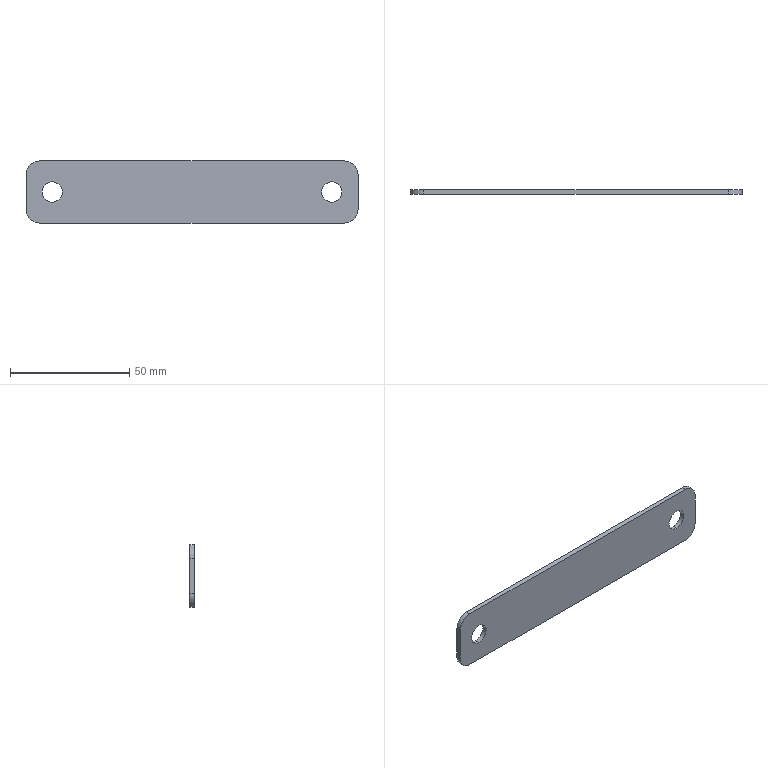Part | STEP file | upcnat117_2_03 | 1 solid | 14 faces | box 139 x 2 x 26 mm | volume 6946 mm3 | cylinder 8 | plane 6 | commonest cylinder face diameters 8.5 x4 11.333 x4
STEP:
#1=CARTESIAN_POINT('',(0.,0.,0.));
#2=DIRECTION('',(0.,0.,1.));
#3=DIRECTION('',(1.,0.,0.));
#4=AXIS2_PLACEMENT_3D('',#1,#2,#3);
#5=CARTESIAN_POINT('',(-58.5,2.,-4.25));
#6=VERTEX_POINT('',#5);
#7=CARTESIAN_POINT('',(-58.5,0.,-4.25));
#8=VERTEX_POINT('',#7);
#9=CARTESIAN_POINT('',(-58.5,0.,-4.25));
#10=DIRECTION('',(0.,-1.,0.));
#11=VECTOR('',#10,1.);
#12=LINE('',#9,#11);
#13=CARTESIAN_POINT('',(-58.5,0.,0.));
#14=DIRECTION('',(0.,-1.,0.));
#15=DIRECTION('',(0.,0.,-1.));
#16=AXIS2_PLACEMENT_3D('',#13,#14,#15);
#17=CYLINDRICAL_SURFACE('',#16,4.25);
#18=CARTESIAN_POINT('',(6.283,0.));
#19=DIRECTION('',(0.,1.));
#20=VECTOR('',#19,1.);
#21=LINE('',#18,#20);
#22=(GEOMETRIC_REPRESENTATION_CONTEXT(2)PARAMETRIC_REPRESENTATION_CONTEXT()REPRESENTATION_CONTEXT('',''));
#23=DEFINITIONAL_REPRESENTATION('',(#21),#22);
#24=PCURVE('',#17,#23);
#25=CARTESIAN_POINT('',(-58.5,0.,0.));
#26=DIRECTION('',(0.,-1.,0.));
#27=DIRECTION('',(0.,0.,-1.));
#28=AXIS2_PLACEMENT_3D('',#25,#26,#27);
#29=CYLINDRICAL_SURFACE('',#28,4.25);
#30=CARTESIAN_POINT('',(0.,0.));
#31=DIRECTION('',(0.,1.));
#32=VECTOR('',#31,1.);
#33=LINE('',#30,#32);
#34=(GEOMETRIC_REPRESENTATION_CONTEXT(2)PARAMETRIC_REPRESENTATION_CONTEXT()REPRESENTATION_CONTEXT('',''));
#35=DEFINITIONAL_REPRESENTATION('',(#33),#34);
#36=PCURVE('',#29,#35);
#37=SURFACE_CURVE('',#12,(#24,#36),.PCURVE_S1.);
#38=EDGE_CURVE('',#6,#8,#37,.T.);
#39=ORIENTED_EDGE('',*,*,#38,.T.);
#40=CARTESIAN_POINT('',(-58.5,0.,4.25));
#41=VERTEX_POINT('',#40);
#42=CARTESIAN_POINT('',(-58.5,0.,0.));
#43=DIRECTION('',(0.,1.,0.));
#44=DIRECTION('',(0.,0.,-1.));
#45=AXIS2_PLACEMENT_3D('',#42,#43,#44);
#46=CIRCLE('',#45,4.25);
#47=CARTESIAN_POINT('',(6.283,0.));
#48=DIRECTION('',(-1.,0.));
#49=VECTOR('',#48,1.);
#50=LINE('',#47,#49);
#51=(GEOMETRIC_REPRESENTATION_CONTEXT(2)PARAMETRIC_REPRESENTATION_CONTEXT()REPRESENTATION_CONTEXT('',''));
#52=DEFINITIONAL_REPRESENTATION('',(#50),#51);
#53=PCURVE('',#17,#52);
#54=CARTESIAN_POINT('',(0.,0.,0.));
#55=DIRECTION('',(0.,1.,0.));
#56=DIRECTION('',(0.,0.,1.));
#57=AXIS2_PLACEMENT_3D('',#54,#55,#56);
#58=PLANE('',#57);
#59=CARTESIAN_POINT('',(0.,-58.5));
#60=DIRECTION('',(-1.,0.));
#61=AXIS2_PLACEMENT_2D('',#59,#60);
#62=CIRCLE('',#61,4.25);
#63=(GEOMETRIC_REPRESENTATION_CONTEXT(2)PARAMETRIC_REPRESENTATION_CONTEXT()REPRESENTATION_CONTEXT('',''));
#64=DEFINITIONAL_REPRESENTATION('',(#62),#63);
#65=PCURVE('',#58,#64);
#66=SURFACE_CURVE('',#46,(#53,#65),.PCURVE_S1.);
#67=EDGE_CURVE('',#8,#41,#66,.T.);
#68=ORIENTED_EDGE('',*,*,#67,.T.);
#69=CARTESIAN_POINT('',(-58.5,2.,4.25));
#70=VERTEX_POINT('',#69);
#71=CARTESIAN_POINT('',(-58.5,0.,4.25));
#72=DIRECTION('',(0.,-1.,0.));
#73=VECTOR('',#72,1.);
#74=LINE('',#71,#73);
#75=CARTESIAN_POINT('',(3.142,0.));
#76=DIRECTION('',(0.,1.));
#77=VECTOR('',#76,1.);
#78=LINE('',#75,#77);
#79=(GEOMETRIC_REPRESENTATION_CONTEXT(2)PARAMETRIC_REPRESENTATION_CONTEXT()REPRESENTATION_CONTEXT('',''));
#80=DEFINITIONAL_REPRESENTATION('',(#78),#79);
#81=PCURVE('',#17,#80);
#82=CARTESIAN_POINT('',(3.142,0.));
#83=DIRECTION('',(0.,1.));
#84=VECTOR('',#83,1.);
#85=LINE('',#82,#84);
#86=(GEOMETRIC_REPRESENTATION_CONTEXT(2)PARAMETRIC_REPRESENTATION_CONTEXT()REPRESENTATION_CONTEXT('',''));
#87=DEFINITIONAL_REPRESENTATION('',(#85),#86);
#88=PCURVE('',#29,#87);
#89=SURFACE_CURVE('',#74,(#81,#88),.PCURVE_S1.);
#90=EDGE_CURVE('',#70,#41,#89,.T.);
#91=ORIENTED_EDGE('',*,*,#90,.F.);
#92=CARTESIAN_POINT('',(-58.5,2.,0.));
#93=DIRECTION('',(0.,-1.,0.));
#94=DIRECTION('',(0.,0.,-1.));
#95=AXIS2_PLACEMENT_3D('',#92,#93,#94);
#96=CIRCLE('',#95,4.25);
#97=CARTESIAN_POINT('',(0.,-2.));
#98=DIRECTION('',(1.,0.));
#99=VECTOR('',#98,1.);
#100=LINE('',#97,#99);
#101=(GEOMETRIC_REPRESENTATION_CONTEXT(2)PARAMETRIC_REPRESENTATION_CONTEXT()REPRESENTATION_CONTEXT('',''));
#102=DEFINITIONAL_REPRESENTATION('',(#100),#101);
#103=PCURVE('',#17,#102);
#104=CARTESIAN_POINT('',(0.,2.,0.));
#105=DIRECTION('',(0.,1.,0.));
#106=DIRECTION('',(0.,0.,1.));
#107=AXIS2_PLACEMENT_3D('',#104,#105,#106);
#108=PLANE('',#107);
#109=CARTESIAN_POINT('',(-4.25,-58.5));
#110=CARTESIAN_POINT('',(-4.25,-51.139));
#111=CARTESIAN_POINT('',(2.125,-54.819));
#112=CARTESIAN_POINT('',(8.5,-58.5));
#113=CARTESIAN_POINT('',(2.125,-62.181));
#114=CARTESIAN_POINT('',(-4.25,-65.861));
#115=CARTESIAN_POINT('',(-4.25,-58.5));
#116=(BOUNDED_CURVE()B_SPLINE_CURVE(2,(#109,#110,#111,#112,#113,#114,#115),.UNSPECIFIED.,.T.,.F.)B_SPLINE_CURVE_WITH_KNOTS((1,2,2,2,2,1),(-2.094,0.,2.094,4.189,6.283,8.378),.UNSPECIFIED.)CURVE()GEOMETRIC_REPRESENTATION_ITEM()RATIONAL_B_SPLINE_CURVE((1.,0.5,1.,0.5,1.,0.5,1.))REPRESENTATION_ITEM(''));
#117=(GEOMETRIC_REPRESENTATION_CONTEXT(2)PARAMETRIC_REPRESENTATION_CONTEXT()REPRESENTATION_CONTEXT('',''));
#118=DEFINITIONAL_REPRESENTATION('',(#116),#117);
#119=PCURVE('',#108,#118);
#120=SURFACE_CURVE('',#96,(#103,#119),.PCURVE_S1.);
#121=EDGE_CURVE('',#70,#6,#120,.T.);
#122=ORIENTED_EDGE('',*,*,#121,.T.);
#123=EDGE_LOOP('',(#39,#68,#91,#122));
#124=FACE_BOUND('',#123,.F.);
#125=ADVANCED_FACE('',(#124),#17,.F.);
#126=CARTESIAN_POINT('',(58.5,2.,-4.25));
#127=VERTEX_POINT('',#126);
#128=CARTESIAN_POINT('',(58.5,0.,-4.25));
#129=VERTEX_POINT('',#128);
#130=CARTESIAN_POINT('',(58.5,0.,-4.25));
#131=DIRECTION('',(0.,-1.,0.));
#132=VECTOR('',#131,1.);
#133=LINE('',#130,#132);
#134=CARTESIAN_POINT('',(58.5,0.,0.));
#135=DIRECTION('',(0.,-1.,0.));
#136=DIRECTION('',(0.,0.,-1.));
#137=AXIS2_PLACEMENT_3D('',#134,#135,#136);
#138=CYLINDRICAL_SURFACE('',#137,4.25);
#139=CARTESIAN_POINT('',(6.283,0.));
#140=DIRECTION('',(0.,1.));
#141=VECTOR('',#140,1.);
#142=LINE('',#139,#141);
#143=(GEOMETRIC_REPRESENTATION_CONTEXT(2)PARAMETRIC_REPRESENTATION_CONTEXT()REPRESENTATION_CONTEXT('',''));
#144=DEFINITIONAL_REPRESENTATION('',(#142),#143);
#145=PCURVE('',#138,#144);
#146=CARTESIAN_POINT('',(58.5,0.,0.));
#147=DIRECTION('',(0.,-1.,0.));
#148=DIRECTION('',(0.,0.,-1.));
#149=AXIS2_PLACEMENT_3D('',#146,#147,#148);
#150=CYLINDRICAL_SURFACE('',#149,4.25);
#151=CARTESIAN_POINT('',(0.,0.));
#152=DIRECTION('',(0.,1.));
#153=VECTOR('',#152,1.);
#154=LINE('',#151,#153);
#155=(GEOMETRIC_REPRESENTATION_CONTEXT(2)PARAMETRIC_REPRESENTATION_CONTEXT()REPRESENTATION_CONTEXT('',''));
#156=DEFINITIONAL_REPRESENTATION('',(#154),#155);
#157=PCURVE('',#150,#156);
#158=SURFACE_CURVE('',#133,(#145,#157),.PCURVE_S1.);
#159=EDGE_CURVE('',#127,#129,#158,.T.);
#160=ORIENTED_EDGE('',*,*,#159,.T.);
#161=CARTESIAN_POINT('',(58.5,0.,4.25));
#162=VERTEX_POINT('',#161);
#163=CARTESIAN_POINT('',(58.5,0.,0.));
#164=DIRECTION('',(0.,1.,0.));
#165=DIRECTION('',(0.,0.,-1.));
#166=AXIS2_PLACEMENT_3D('',#163,#164,#165);
#167=CIRCLE('',#166,4.25);
#168=CARTESIAN_POINT('',(6.283,0.));
#169=DIRECTION('',(-1.,0.));
#170=VECTOR('',#169,1.);
#171=LINE('',#168,#170);
#172=(GEOMETRIC_REPRESENTATION_CONTEXT(2)PARAMETRIC_REPRESENTATION_CONTEXT()REPRESENTATION_CONTEXT('',''));
#173=DEFINITIONAL_REPRESENTATION('',(#171),#172);
#174=PCURVE('',#138,#173);
#175=CARTESIAN_POINT('',(0.,58.5));
#176=DIRECTION('',(-1.,0.));
#177=AXIS2_PLACEMENT_2D('',#175,#176);
#178=CIRCLE('',#177,4.25);
#179=(GEOMETRIC_REPRESENTATION_CONTEXT(2)PARAMETRIC_REPRESENTATION_CONTEXT()REPRESENTATION_CONTEXT('',''));
#180=DEFINITIONAL_REPRESENTATION('',(#178),#179);
#181=PCURVE('',#58,#180);
#182=SURFACE_CURVE('',#167,(#174,#181),.PCURVE_S1.);
#183=EDGE_CURVE('',#129,#162,#182,.T.);
#184=ORIENTED_EDGE('',*,*,#183,.T.);
#185=CARTESIAN_POINT('',(58.5,2.,4.25));
#186=VERTEX_POINT('',#185);
#187=CARTESIAN_POINT('',(58.5,0.,4.25));
#188=DIRECTION('',(0.,-1.,0.));
#189=VECTOR('',#188,1.);
#190=LINE('',#187,#189);
#191=CARTESIAN_POINT('',(3.142,0.));
#192=DIRECTION('',(0.,1.));
#193=VECTOR('',#192,1.);
#194=LINE('',#191,#193);
#195=(GEOMETRIC_REPRESENTATION_CONTEXT(2)PARAMETRIC_REPRESENTATION_CONTEXT()REPRESENTATION_CONTEXT('',''));
#196=DEFINITIONAL_REPRESENTATION('',(#194),#195);
#197=PCURVE('',#138,#196);
#198=CARTESIAN_POINT('',(3.142,0.));
#199=DIRECTION('',(0.,1.));
#200=VECTOR('',#199,1.);
#201=LINE('',#198,#200);
#202=(GEOMETRIC_REPRESENTATION_CONTEXT(2)PARAMETRIC_REPRESENTATION_CONTEXT()REPRESENTATION_CONTEXT('',''));
#203=DEFINITIONAL_REPRESENTATION('',(#201),#202);
#204=PCURVE('',#150,#203);
#205=SURFACE_CURVE('',#190,(#197,#204),.PCURVE_S1.);
#206=EDGE_CURVE('',#186,#162,#205,.T.);
#207=ORIENTED_EDGE('',*,*,#206,.F.);
#208=CARTESIAN_POINT('',(58.5,2.,0.));
#209=DIRECTION('',(0.,-1.,0.));
#210=DIRECTION('',(0.,0.,-1.));
#211=AXIS2_PLACEMENT_3D('',#208,#209,#210);
#212=CIRCLE('',#211,4.25);
#213=CARTESIAN_POINT('',(0.,-2.));
#214=DIRECTION('',(1.,0.));
#215=VECTOR('',#214,1.);
#216=LINE('',#213,#215);
#217=(GEOMETRIC_REPRESENTATION_CONTEXT(2)PARAMETRIC_REPRESENTATION_CONTEXT()REPRESENTATION_CONTEXT('',''));
#218=DEFINITIONAL_REPRESENTATION('',(#216),#217);
#219=PCURVE('',#138,#218);
#220=CARTESIAN_POINT('',(-4.25,58.5));
#221=CARTESIAN_POINT('',(-4.25,65.861));
#222=CARTESIAN_POINT('',(2.125,62.181));
#223=CARTESIAN_POINT('',(8.5,58.5));
#224=CARTESIAN_POINT('',(2.125,54.819));
#225=CARTESIAN_POINT('',(-4.25,51.139));
#226=CARTESIAN_POINT('',(-4.25,58.5));
#227=(BOUNDED_CURVE()B_SPLINE_CURVE(2,(#220,#221,#222,#223,#224,#225,#226),.UNSPECIFIED.,.T.,.F.)B_SPLINE_CURVE_WITH_KNOTS((1,2,2,2,2,1),(-2.094,0.,2.094,4.189,6.283,8.378),.UNSPECIFIED.)CURVE()GEOMETRIC_REPRESENTATION_ITEM()RATIONAL_B_SPLINE_CURVE((1.,0.5,1.,0.5,1.,0.5,1.))REPRESENTATION_ITEM(''));
#228=(GEOMETRIC_REPRESENTATION_CONTEXT(2)PARAMETRIC_REPRESENTATION_CONTEXT()REPRESENTATION_CONTEXT('',''));
#229=DEFINITIONAL_REPRESENTATION('',(#227),#228);
#230=PCURVE('',#108,#229);
#231=SURFACE_CURVE('',#212,(#219,#230),.PCURVE_S1.);
#232=EDGE_CURVE('',#186,#127,#231,.T.);
#233=ORIENTED_EDGE('',*,*,#232,.T.);
#234=EDGE_LOOP('',(#160,#184,#207,#233));
#235=FACE_BOUND('',#234,.F.);
#236=ADVANCED_FACE('',(#235),#138,.F.);
#237=CARTESIAN_POINT('',(-58.5,2.,0.));
#238=DIRECTION('',(0.,-1.,0.));
#239=DIRECTION('',(0.,0.,-1.));
#240=AXIS2_PLACEMENT_3D('',#237,#238,#239);
#241=CIRCLE('',#240,4.25);
#242=CARTESIAN_POINT('',(-4.25,-58.5));
#243=CARTESIAN_POINT('',(-4.25,-51.139));
#244=CARTESIAN_POINT('',(2.125,-54.819));
#245=CARTESIAN_POINT('',(8.5,-58.5));
#246=CARTESIAN_POINT('',(2.125,-62.181));
#247=CARTESIAN_POINT('',(-4.25,-65.861));
#248=CARTESIAN_POINT('',(-4.25,-58.5));
#249=(BOUNDED_CURVE()B_SPLINE_CURVE(2,(#242,#243,#244,#245,#246,#247,#248),.UNSPECIFIED.,.T.,.F.)B_SPLINE_CURVE_WITH_KNOTS((1,2,2,2,2,1),(-2.094,0.,2.094,4.189,6.283,8.378),.UNSPECIFIED.)CURVE()GEOMETRIC_REPRESENTATION_ITEM()RATIONAL_B_SPLINE_CURVE((1.,0.5,1.,0.5,1.,0.5,1.))REPRESENTATION_ITEM(''));
#250=(GEOMETRIC_REPRESENTATION_CONTEXT(2)PARAMETRIC_REPRESENTATION_CONTEXT()REPRESENTATION_CONTEXT('',''));
#251=DEFINITIONAL_REPRESENTATION('',(#249),#250);
#252=PCURVE('',#108,#251);
#253=CARTESIAN_POINT('',(0.,-2.));
#254=DIRECTION('',(1.,0.));
#255=VECTOR('',#254,1.);
#256=LINE('',#253,#255);
#257=(GEOMETRIC_REPRESENTATION_CONTEXT(2)PARAMETRIC_REPRESENTATION_CONTEXT()REPRESENTATION_CONTEXT('',''));
#258=DEFINITIONAL_REPRESENTATION('',(#256),#257);
#259=PCURVE('',#29,#258);
#260=SURFACE_CURVE('',#241,(#252,#259),.PCURVE_S1.);
#261=EDGE_CURVE('',#6,#70,#260,.T.);
#262=ORIENTED_EDGE('',*,*,#261,.T.);
#263=ORIENTED_EDGE('',*,*,#121,.T.);
#264=EDGE_LOOP('',(#262,#263));
#265=FACE_BOUND('',#264,.T.);
#266=CARTESIAN_POINT('',(58.5,2.,0.));
#267=DIRECTION('',(0.,-1.,0.));
#268=DIRECTION('',(0.,0.,-1.));
#269=AXIS2_PLACEMENT_3D('',#266,#267,#268);
#270=CIRCLE('',#269,4.25);
#271=CARTESIAN_POINT('',(-4.25,58.5));
#272=CARTESIAN_POINT('',(-4.25,65.861));
#273=CARTESIAN_POINT('',(2.125,62.181));
#274=CARTESIAN_POINT('',(8.5,58.5));
#275=CARTESIAN_POINT('',(2.125,54.819));
#276=CARTESIAN_POINT('',(-4.25,51.139));
#277=CARTESIAN_POINT('',(-4.25,58.5));
#278=(BOUNDED_CURVE()B_SPLINE_CURVE(2,(#271,#272,#273,#274,#275,#276,#277),.UNSPECIFIED.,.T.,.F.)B_SPLINE_CURVE_WITH_KNOTS((1,2,2,2,2,1),(-2.094,0.,2.094,4.189,6.283,8.378),.UNSPECIFIED.)CURVE()GEOMETRIC_REPRESENTATION_ITEM()RATIONAL_B_SPLINE_CURVE((1.,0.5,1.,0.5,1.,0.5,1.))REPRESENTATION_ITEM(''));
#279=(GEOMETRIC_REPRESENTATION_CONTEXT(2)PARAMETRIC_REPRESENTATION_CONTEXT()REPRESENTATION_CONTEXT('',''));
#280=DEFINITIONAL_REPRESENTATION('',(#278),#279);
#281=PCURVE('',#108,#280);
#282=CARTESIAN_POINT('',(0.,-2.));
#283=DIRECTION('',(1.,0.));
#284=VECTOR('',#283,1.);
#285=LINE('',#282,#284);
#286=(GEOMETRIC_REPRESENTATION_CONTEXT(2)PARAMETRIC_REPRESENTATION_CONTEXT()REPRESENTATION_CONTEXT('',''));
#287=DEFINITIONAL_REPRESENTATION('',(#285),#286);
#288=PCURVE('',#150,#287);
#289=SURFACE_CURVE('',#270,(#281,#288),.PCURVE_S1.);
#290=EDGE_CURVE('',#127,#186,#289,.T.);
#291=ORIENTED_EDGE('',*,*,#290,.T.);
#292=ORIENTED_EDGE('',*,*,#232,.T.);
#293=EDGE_LOOP('',(#291,#292));
#294=FACE_BOUND('',#293,.T.);
#295=CARTESIAN_POINT('',(63.833,2.,-13.));
#296=VERTEX_POINT('',#295);
#297=CARTESIAN_POINT('',(-63.833,2.,-13.));
#298=VERTEX_POINT('',#297);
#299=CARTESIAN_POINT('',(0.,2.,-13.));
#300=DIRECTION('',(-1.,0.,0.));
#301=VECTOR('',#300,1.);
#302=LINE('',#299,#301);
#303=CARTESIAN_POINT('',(-13.,0.));
#304=DIRECTION('',(0.,-1.));
#305=VECTOR('',#304,1.);
#306=LINE('',#303,#305);
#307=(GEOMETRIC_REPRESENTATION_CONTEXT(2)PARAMETRIC_REPRESENTATION_CONTEXT()REPRESENTATION_CONTEXT('',''));
#308=DEFINITIONAL_REPRESENTATION('',(#306),#307);
#309=PCURVE('',#108,#308);
#310=CARTESIAN_POINT('',(-63.833,0.,-13.));
#311=DIRECTION('',(0.,0.,-1.));
#312=DIRECTION('',(-1.,0.,0.));
#313=AXIS2_PLACEMENT_3D('',#310,#311,#312);
#314=PLANE('',#313);
#315=CARTESIAN_POINT('',(-63.833,2.));
#316=DIRECTION('',(1.,0.));
#317=VECTOR('',#316,1.);
#318=LINE('',#315,#317);
#319=(GEOMETRIC_REPRESENTATION_CONTEXT(2)PARAMETRIC_REPRESENTATION_CONTEXT()REPRESENTATION_CONTEXT('',''));
#320=DEFINITIONAL_REPRESENTATION('',(#318),#319);
#321=PCURVE('',#314,#320);
#322=SURFACE_CURVE('',#302,(#309,#321),.PCURVE_S1.);
#323=EDGE_CURVE('',#296,#298,#322,.T.);
#324=ORIENTED_EDGE('',*,*,#323,.T.);
#325=CARTESIAN_POINT('',(-69.5,2.,-7.333));
#326=VERTEX_POINT('',#325);
#327=CARTESIAN_POINT('',(-63.833,2.,-7.333));
#328=DIRECTION('',(0.,1.,0.));
#329=DIRECTION('',(0.,0.,-1.));
#330=AXIS2_PLACEMENT_3D('',#327,#328,#329);
#331=CIRCLE('',#330,5.667);
#332=CARTESIAN_POINT('',(-7.333,-63.833));
#333=DIRECTION('',(-1.,0.));
#334=AXIS2_PLACEMENT_2D('',#332,#333);
#335=CIRCLE('',#334,5.667);
#336=(GEOMETRIC_REPRESENTATION_CONTEXT(2)PARAMETRIC_REPRESENTATION_CONTEXT()REPRESENTATION_CONTEXT('',''));
#337=DEFINITIONAL_REPRESENTATION('',(#335),#336);
#338=PCURVE('',#108,#337);
#339=CARTESIAN_POINT('',(-63.833,0.,-7.333));
#340=DIRECTION('',(0.,-1.,0.));
#341=DIRECTION('',(0.,0.,-1.));
#342=AXIS2_PLACEMENT_3D('',#339,#340,#341);
#343=CYLINDRICAL_SURFACE('',#342,5.667);
#344=CARTESIAN_POINT('',(6.283,-2.));
#345=DIRECTION('',(-1.,0.));
#346=VECTOR('',#345,1.);
#347=LINE('',#344,#346);
#348=(GEOMETRIC_REPRESENTATION_CONTEXT(2)PARAMETRIC_REPRESENTATION_CONTEXT()REPRESENTATION_CONTEXT('',''));
#349=DEFINITIONAL_REPRESENTATION('',(#347),#348);
#350=PCURVE('',#343,#349);
#351=SURFACE_CURVE('',#331,(#338,#350),.PCURVE_S1.);
#352=EDGE_CURVE('',#298,#326,#351,.T.);
#353=ORIENTED_EDGE('',*,*,#352,.T.);
#354=CARTESIAN_POINT('',(-69.5,2.,7.333));
#355=VERTEX_POINT('',#354);
#356=CARTESIAN_POINT('',(-69.5,2.,0.));
#357=DIRECTION('',(0.,0.,1.));
#358=VECTOR('',#357,1.);
#359=LINE('',#356,#358);
#360=CARTESIAN_POINT('',(0.,-69.5));
#361=DIRECTION('',(1.,0.));
#362=VECTOR('',#361,1.);
#363=LINE('',#360,#362);
#364=(GEOMETRIC_REPRESENTATION_CONTEXT(2)PARAMETRIC_REPRESENTATION_CONTEXT()REPRESENTATION_CONTEXT('',''));
#365=DEFINITIONAL_REPRESENTATION('',(#363),#364);
#366=PCURVE('',#108,#365);
#367=CARTESIAN_POINT('',(-69.5,0.,7.333));
#368=DIRECTION('',(-1.,0.,0.));
#369=DIRECTION('',(0.,0.,1.));
#370=AXIS2_PLACEMENT_3D('',#367,#368,#369);
#371=PLANE('',#370);
#372=CARTESIAN_POINT('',(-7.333,2.));
#373=DIRECTION('',(1.,0.));
#374=VECTOR('',#373,1.);
#375=LINE('',#372,#374);
#376=(GEOMETRIC_REPRESENTATION_CONTEXT(2)PARAMETRIC_REPRESENTATION_CONTEXT()REPRESENTATION_CONTEXT('',''));
#377=DEFINITIONAL_REPRESENTATION('',(#375),#376);
#378=PCURVE('',#371,#377);
#379=SURFACE_CURVE('',#359,(#366,#378),.PCURVE_S1.);
#380=EDGE_CURVE('',#326,#355,#379,.T.);
#381=ORIENTED_EDGE('',*,*,#380,.T.);
#382=CARTESIAN_POINT('',(-63.833,2.,13.));
#383=VERTEX_POINT('',#382);
#384=CARTESIAN_POINT('',(-63.833,2.,7.333));
#385=DIRECTION('',(0.,1.,0.));
#386=DIRECTION('',(0.,0.,-1.));
#387=AXIS2_PLACEMENT_3D('',#384,#385,#386);
#388=CIRCLE('',#387,5.667);
#389=CARTESIAN_POINT('',(7.333,-63.833));
#390=DIRECTION('',(-1.,0.));
#391=AXIS2_PLACEMENT_2D('',#389,#390);
#392=CIRCLE('',#391,5.667);
#393=(GEOMETRIC_REPRESENTATION_CONTEXT(2)PARAMETRIC_REPRESENTATION_CONTEXT()REPRESENTATION_CONTEXT('',''));
#394=DEFINITIONAL_REPRESENTATION('',(#392),#393);
#395=PCURVE('',#108,#394);
#396=CARTESIAN_POINT('',(-63.833,0.,7.333));
#397=DIRECTION('',(0.,-1.,0.));
#398=DIRECTION('',(0.,0.,-1.));
#399=AXIS2_PLACEMENT_3D('',#396,#397,#398);
#400=CYLINDRICAL_SURFACE('',#399,5.667);
#401=CARTESIAN_POINT('',(6.283,-2.));
#402=DIRECTION('',(-1.,0.));
#403=VECTOR('',#402,1.);
#404=LINE('',#401,#403);
#405=(GEOMETRIC_REPRESENTATION_CONTEXT(2)PARAMETRIC_REPRESENTATION_CONTEXT()REPRESENTATION_CONTEXT('',''));
#406=DEFINITIONAL_REPRESENTATION('',(#404),#405);
#407=PCURVE('',#400,#406);
#408=SURFACE_CURVE('',#388,(#395,#407),.PCURVE_S1.);
#409=EDGE_CURVE('',#355,#383,#408,.T.);
#410=ORIENTED_EDGE('',*,*,#409,.T.);
#411=CARTESIAN_POINT('',(63.833,2.,13.));
#412=VERTEX_POINT('',#411);
#413=CARTESIAN_POINT('',(0.,2.,13.));
#414=DIRECTION('',(1.,0.,0.));
#415=VECTOR('',#414,1.);
#416=LINE('',#413,#415);
#417=CARTESIAN_POINT('',(13.,0.));
#418=DIRECTION('',(0.,1.));
#419=VECTOR('',#418,1.);
#420=LINE('',#417,#419);
#421=(GEOMETRIC_REPRESENTATION_CONTEXT(2)PARAMETRIC_REPRESENTATION_CONTEXT()REPRESENTATION_CONTEXT('',''));
#422=DEFINITIONAL_REPRESENTATION('',(#420),#421);
#423=PCURVE('',#108,#422);
#424=CARTESIAN_POINT('',(63.833,0.,13.));
#425=DIRECTION('',(0.,0.,1.));
#426=DIRECTION('',(1.,0.,0.));
#427=AXIS2_PLACEMENT_3D('',#424,#425,#426);
#428=PLANE('',#427);
#429=CARTESIAN_POINT('',(-63.833,2.));
#430=DIRECTION('',(1.,0.));
#431=VECTOR('',#430,1.);
#432=LINE('',#429,#431);
#433=(GEOMETRIC_REPRESENTATION_CONTEXT(2)PARAMETRIC_REPRESENTATION_CONTEXT()REPRESENTATION_CONTEXT('',''));
#434=DEFINITIONAL_REPRESENTATION('',(#432),#433);
#435=PCURVE('',#428,#434);
#436=SURFACE_CURVE('',#416,(#423,#435),.PCURVE_S1.);
#437=EDGE_CURVE('',#383,#412,#436,.T.);
#438=ORIENTED_EDGE('',*,*,#437,.T.);
#439=CARTESIAN_POINT('',(69.5,2.,7.333));
#440=VERTEX_POINT('',#439);
#441=CARTESIAN_POINT('',(63.833,2.,7.333));
#442=DIRECTION('',(0.,1.,0.));
#443=DIRECTION('',(0.,0.,-1.));
#444=AXIS2_PLACEMENT_3D('',#441,#442,#443);
#445=CIRCLE('',#444,5.667);
#446=CARTESIAN_POINT('',(7.333,63.833));
#447=DIRECTION('',(-1.,0.));
#448=AXIS2_PLACEMENT_2D('',#446,#447);
#449=CIRCLE('',#448,5.667);
#450=(GEOMETRIC_REPRESENTATION_CONTEXT(2)PARAMETRIC_REPRESENTATION_CONTEXT()REPRESENTATION_CONTEXT('',''));
#451=DEFINITIONAL_REPRESENTATION('',(#449),#450);
#452=PCURVE('',#108,#451);
#453=CARTESIAN_POINT('',(63.833,0.,7.333));
#454=DIRECTION('',(0.,-1.,0.));
#455=DIRECTION('',(0.,0.,-1.));
#456=AXIS2_PLACEMENT_3D('',#453,#454,#455);
#457=CYLINDRICAL_SURFACE('',#456,5.667);
#458=CARTESIAN_POINT('',(6.283,-2.));
#459=DIRECTION('',(-1.,0.));
#460=VECTOR('',#459,1.);
#461=LINE('',#458,#460);
#462=(GEOMETRIC_REPRESENTATION_CONTEXT(2)PARAMETRIC_REPRESENTATION_CONTEXT()REPRESENTATION_CONTEXT('',''));
#463=DEFINITIONAL_REPRESENTATION('',(#461),#462);
#464=PCURVE('',#457,#463);
#465=SURFACE_CURVE('',#445,(#452,#464),.PCURVE_S1.);
#466=EDGE_CURVE('',#412,#440,#465,.T.);
#467=ORIENTED_EDGE('',*,*,#466,.T.);
#468=CARTESIAN_POINT('',(69.5,2.,-7.333));
#469=VERTEX_POINT('',#468);
#470=CARTESIAN_POINT('',(69.5,2.,0.));
#471=DIRECTION('',(0.,0.,-1.));
#472=VECTOR('',#471,1.);
#473=LINE('',#470,#472);
#474=CARTESIAN_POINT('',(0.,69.5));
#475=DIRECTION('',(-1.,0.));
#476=VECTOR('',#475,1.);
#477=LINE('',#474,#476);
#478=(GEOMETRIC_REPRESENTATION_CONTEXT(2)PARAMETRIC_REPRESENTATION_CONTEXT()REPRESENTATION_CONTEXT('',''));
#479=DEFINITIONAL_REPRESENTATION('',(#477),#478);
#480=PCURVE('',#108,#479);
#481=CARTESIAN_POINT('',(69.5,0.,-7.333));
#482=DIRECTION('',(1.,0.,0.));
#483=DIRECTION('',(0.,0.,-1.));
#484=AXIS2_PLACEMENT_3D('',#481,#482,#483);
#485=PLANE('',#484);
#486=CARTESIAN_POINT('',(-7.333,2.));
#487=DIRECTION('',(1.,0.));
#488=VECTOR('',#487,1.);
#489=LINE('',#486,#488);
#490=(GEOMETRIC_REPRESENTATION_CONTEXT(2)PARAMETRIC_REPRESENTATION_CONTEXT()REPRESENTATION_CONTEXT('',''));
#491=DEFINITIONAL_REPRESENTATION('',(#489),#490);
#492=PCURVE('',#485,#491);
#493=SURFACE_CURVE('',#473,(#480,#492),.PCURVE_S1.);
#494=EDGE_CURVE('',#440,#469,#493,.T.);
#495=ORIENTED_EDGE('',*,*,#494,.T.);
#496=CARTESIAN_POINT('',(63.833,2.,-7.333));
#497=DIRECTION('',(0.,1.,0.));
#498=DIRECTION('',(0.,0.,-1.));
#499=AXIS2_PLACEMENT_3D('',#496,#497,#498);
#500=CIRCLE('',#499,5.667);
#501=CARTESIAN_POINT('',(-7.333,63.833));
#502=DIRECTION('',(-1.,0.));
#503=AXIS2_PLACEMENT_2D('',#501,#502);
#504=CIRCLE('',#503,5.667);
#505=(GEOMETRIC_REPRESENTATION_CONTEXT(2)PARAMETRIC_REPRESENTATION_CONTEXT()REPRESENTATION_CONTEXT('',''));
#506=DEFINITIONAL_REPRESENTATION('',(#504),#505);
#507=PCURVE('',#108,#506);
#508=CARTESIAN_POINT('',(63.833,0.,-7.333));
#509=DIRECTION('',(0.,-1.,0.));
#510=DIRECTION('',(0.,0.,-1.));
#511=AXIS2_PLACEMENT_3D('',#508,#509,#510);
#512=CYLINDRICAL_SURFACE('',#511,5.667);
#513=CARTESIAN_POINT('',(6.283,-2.));
#514=DIRECTION('',(-1.,0.));
#515=VECTOR('',#514,1.);
#516=LINE('',#513,#515);
#517=(GEOMETRIC_REPRESENTATION_CONTEXT(2)PARAMETRIC_REPRESENTATION_CONTEXT()REPRESENTATION_CONTEXT('',''));
#518=DEFINITIONAL_REPRESENTATION('',(#516),#517);
#519=PCURVE('',#512,#518);
#520=SURFACE_CURVE('',#500,(#507,#519),.PCURVE_S1.);
#521=EDGE_CURVE('',#469,#296,#520,.T.);
#522=ORIENTED_EDGE('',*,*,#521,.T.);
#523=EDGE_LOOP('',(#324,#353,#381,#410,#438,#467,#495,#522));
#524=FACE_BOUND('',#523,.T.);
#525=ADVANCED_FACE('',(#265,#294,#524),#108,.T.);
#526=CARTESIAN_POINT('',(-58.5,0.,0.));
#527=DIRECTION('',(0.,1.,0.));
#528=DIRECTION('',(0.,0.,-1.));
#529=AXIS2_PLACEMENT_3D('',#526,#527,#528);
#530=CIRCLE('',#529,4.25);
#531=CARTESIAN_POINT('',(6.283,0.));
#532=DIRECTION('',(-1.,0.));
#533=VECTOR('',#532,1.);
#534=LINE('',#531,#533);
#535=(GEOMETRIC_REPRESENTATION_CONTEXT(2)PARAMETRIC_REPRESENTATION_CONTEXT()REPRESENTATION_CONTEXT('',''));
#536=DEFINITIONAL_REPRESENTATION('',(#534),#535);
#537=PCURVE('',#29,#536);
#538=CARTESIAN_POINT('',(0.,-58.5));
#539=DIRECTION('',(-1.,0.));
#540=AXIS2_PLACEMENT_2D('',#538,#539);
#541=CIRCLE('',#540,4.25);
#542=(GEOMETRIC_REPRESENTATION_CONTEXT(2)PARAMETRIC_REPRESENTATION_CONTEXT()REPRESENTATION_CONTEXT('',''));
#543=DEFINITIONAL_REPRESENTATION('',(#541),#542);
#544=PCURVE('',#58,#543);
#545=SURFACE_CURVE('',#530,(#537,#544),.PCURVE_S1.);
#546=EDGE_CURVE('',#41,#8,#545,.T.);
#547=ORIENTED_EDGE('',*,*,#546,.T.);
#548=ORIENTED_EDGE('',*,*,#38,.F.);
#549=ORIENTED_EDGE('',*,*,#261,.T.);
#550=ORIENTED_EDGE('',*,*,#90,.T.);
#551=EDGE_LOOP('',(#547,#548,#549,#550));
#552=FACE_BOUND('',#551,.F.);
#553=ADVANCED_FACE('',(#552),#29,.F.);
#554=CARTESIAN_POINT('',(58.5,0.,0.));
#555=DIRECTION('',(0.,1.,0.));
#556=DIRECTION('',(0.,0.,-1.));
#557=AXIS2_PLACEMENT_3D('',#554,#555,#556);
#558=CIRCLE('',#557,4.25);
#559=CARTESIAN_POINT('',(6.283,0.));
#560=DIRECTION('',(-1.,0.));
#561=VECTOR('',#560,1.);
#562=LINE('',#559,#561);
#563=(GEOMETRIC_REPRESENTATION_CONTEXT(2)PARAMETRIC_REPRESENTATION_CONTEXT()REPRESENTATION_CONTEXT('',''));
#564=DEFINITIONAL_REPRESENTATION('',(#562),#563);
#565=PCURVE('',#150,#564);
#566=CARTESIAN_POINT('',(0.,58.5));
#567=DIRECTION('',(-1.,0.));
#568=AXIS2_PLACEMENT_2D('',#566,#567);
#569=CIRCLE('',#568,4.25);
#570=(GEOMETRIC_REPRESENTATION_CONTEXT(2)PARAMETRIC_REPRESENTATION_CONTEXT()REPRESENTATION_CONTEXT('',''));
#571=DEFINITIONAL_REPRESENTATION('',(#569),#570);
#572=PCURVE('',#58,#571);
#573=SURFACE_CURVE('',#558,(#565,#572),.PCURVE_S1.);
#574=EDGE_CURVE('',#162,#129,#573,.T.);
#575=ORIENTED_EDGE('',*,*,#574,.T.);
#576=ORIENTED_EDGE('',*,*,#159,.F.);
#577=ORIENTED_EDGE('',*,*,#290,.T.);
#578=ORIENTED_EDGE('',*,*,#206,.T.);
#579=EDGE_LOOP('',(#575,#576,#577,#578));
#580=FACE_BOUND('',#579,.F.);
#581=ADVANCED_FACE('',(#580),#150,.F.);
#582=CARTESIAN_POINT('',(-63.833,0.,-13.));
#583=VERTEX_POINT('',#582);
#584=CARTESIAN_POINT('',(-69.5,0.,-7.333));
#585=VERTEX_POINT('',#584);
#586=CARTESIAN_POINT('',(-63.833,0.,-7.333));
#587=DIRECTION('',(0.,1.,0.));
#588=DIRECTION('',(0.,0.,-1.));
#589=AXIS2_PLACEMENT_3D('',#586,#587,#588);
#590=CIRCLE('',#589,5.667);
#591=CARTESIAN_POINT('',(6.283,0.));
#592=DIRECTION('',(-1.,0.));
#593=VECTOR('',#592,1.);
#594=LINE('',#591,#593);
#595=(GEOMETRIC_REPRESENTATION_CONTEXT(2)PARAMETRIC_REPRESENTATION_CONTEXT()REPRESENTATION_CONTEXT('',''));
#596=DEFINITIONAL_REPRESENTATION('',(#594),#595);
#597=PCURVE('',#343,#596);
#598=CARTESIAN_POINT('',(-7.333,-63.833));
#599=DIRECTION('',(-1.,0.));
#600=AXIS2_PLACEMENT_2D('',#598,#599);
#601=CIRCLE('',#600,5.667);
#602=(GEOMETRIC_REPRESENTATION_CONTEXT(2)PARAMETRIC_REPRESENTATION_CONTEXT()REPRESENTATION_CONTEXT('',''));
#603=DEFINITIONAL_REPRESENTATION('',(#601),#602);
#604=PCURVE('',#58,#603);
#605=SURFACE_CURVE('',#590,(#597,#604),.PCURVE_S1.);
#606=EDGE_CURVE('',#583,#585,#605,.T.);
#607=ORIENTED_EDGE('',*,*,#606,.T.);
#608=CARTESIAN_POINT('',(-69.5,0.,-7.333));
#609=DIRECTION('',(0.,1.,0.));
#610=VECTOR('',#609,1.);
#611=LINE('',#608,#610);
#612=CARTESIAN_POINT('',(4.712,0.));
#613=DIRECTION('',(0.,-1.));
#614=VECTOR('',#613,1.);
#615=LINE('',#612,#614);
#616=(GEOMETRIC_REPRESENTATION_CONTEXT(2)PARAMETRIC_REPRESENTATION_CONTEXT()REPRESENTATION_CONTEXT('',''));
#617=DEFINITIONAL_REPRESENTATION('',(#615),#616);
#618=PCURVE('',#343,#617);
#619=CARTESIAN_POINT('',(-14.667,0.));
#620=DIRECTION('',(0.,1.));
#621=VECTOR('',#620,1.);
#622=LINE('',#619,#621);
#623=(GEOMETRIC_REPRESENTATION_CONTEXT(2)PARAMETRIC_REPRESENTATION_CONTEXT()REPRESENTATION_CONTEXT('',''));
#624=DEFINITIONAL_REPRESENTATION('',(#622),#623);
#625=PCURVE('',#371,#624);
#626=SURFACE_CURVE('',#611,(#618,#625),.PCURVE_S1.);
#627=EDGE_CURVE('',#585,#326,#626,.T.);
#628=ORIENTED_EDGE('',*,*,#627,.T.);
#629=ORIENTED_EDGE('',*,*,#352,.F.);
#630=CARTESIAN_POINT('',(-63.833,0.,-13.));
#631=DIRECTION('',(0.,-1.,0.));
#632=VECTOR('',#631,1.);
#633=LINE('',#630,#632);
#634=CARTESIAN_POINT('',(6.283,0.));
#635=DIRECTION('',(0.,1.));
#636=VECTOR('',#635,1.);
#637=LINE('',#634,#636);
#638=(GEOMETRIC_REPRESENTATION_CONTEXT(2)PARAMETRIC_REPRESENTATION_CONTEXT()REPRESENTATION_CONTEXT('',''));
#639=DEFINITIONAL_REPRESENTATION('',(#637),#638);
#640=PCURVE('',#343,#639);
#641=CARTESIAN_POINT('',(0.,0.));
#642=DIRECTION('',(0.,-1.));
#643=VECTOR('',#642,1.);
#644=LINE('',#641,#643);
#645=(GEOMETRIC_REPRESENTATION_CONTEXT(2)PARAMETRIC_REPRESENTATION_CONTEXT()REPRESENTATION_CONTEXT('',''));
#646=DEFINITIONAL_REPRESENTATION('',(#644),#645);
#647=PCURVE('',#314,#646);
#648=SURFACE_CURVE('',#633,(#640,#647),.PCURVE_S1.);
#649=EDGE_CURVE('',#298,#583,#648,.T.);
#650=ORIENTED_EDGE('',*,*,#649,.T.);
#651=EDGE_LOOP('',(#607,#628,#629,#650));
#652=FACE_BOUND('',#651,.T.);
#653=ADVANCED_FACE('',(#652),#343,.T.);
#654=CARTESIAN_POINT('',(63.833,0.,-13.));
#655=VERTEX_POINT('',#654);
#656=CARTESIAN_POINT('',(-63.833,0.,-13.));
#657=DIRECTION('',(-1.,0.,0.));
#658=VECTOR('',#657,1.);
#659=LINE('',#656,#658);
#660=CARTESIAN_POINT('',(0.,0.));
#661=DIRECTION('',(1.,0.));
#662=VECTOR('',#661,1.);
#663=LINE('',#660,#662);
#664=(GEOMETRIC_REPRESENTATION_CONTEXT(2)PARAMETRIC_REPRESENTATION_CONTEXT()REPRESENTATION_CONTEXT('',''));
#665=DEFINITIONAL_REPRESENTATION('',(#663),#664);
#666=PCURVE('',#314,#665);
#667=CARTESIAN_POINT('',(-13.,-63.833));
#668=DIRECTION('',(0.,-1.));
#669=VECTOR('',#668,1.);
#670=LINE('',#667,#669);
#671=(GEOMETRIC_REPRESENTATION_CONTEXT(2)PARAMETRIC_REPRESENTATION_CONTEXT()REPRESENTATION_CONTEXT('',''));
#672=DEFINITIONAL_REPRESENTATION('',(#670),#671);
#673=PCURVE('',#58,#672);
#674=SURFACE_CURVE('',#659,(#666,#673),.PCURVE_S1.);
#675=EDGE_CURVE('',#655,#583,#674,.T.);
#676=ORIENTED_EDGE('',*,*,#675,.T.);
#677=ORIENTED_EDGE('',*,*,#649,.F.);
#678=ORIENTED_EDGE('',*,*,#323,.F.);
#679=CARTESIAN_POINT('',(63.833,0.,-13.));
#680=DIRECTION('',(0.,-1.,0.));
#681=VECTOR('',#680,1.);
#682=LINE('',#679,#681);
#683=CARTESIAN_POINT('',(-127.667,0.));
#684=DIRECTION('',(0.,-1.));
#685=VECTOR('',#684,1.);
#686=LINE('',#683,#685);
#687=(GEOMETRIC_REPRESENTATION_CONTEXT(2)PARAMETRIC_REPRESENTATION_CONTEXT()REPRESENTATION_CONTEXT('',''));
#688=DEFINITIONAL_REPRESENTATION('',(#686),#687);
#689=PCURVE('',#314,#688);
#690=CARTESIAN_POINT('',(0.,0.));
#691=DIRECTION('',(0.,1.));
#692=VECTOR('',#691,1.);
#693=LINE('',#690,#692);
#694=(GEOMETRIC_REPRESENTATION_CONTEXT(2)PARAMETRIC_REPRESENTATION_CONTEXT()REPRESENTATION_CONTEXT('',''));
#695=DEFINITIONAL_REPRESENTATION('',(#693),#694);
#696=PCURVE('',#512,#695);
#697=SURFACE_CURVE('',#682,(#689,#696),.PCURVE_S1.);
#698=EDGE_CURVE('',#296,#655,#697,.T.);
#699=ORIENTED_EDGE('',*,*,#698,.T.);
#700=EDGE_LOOP('',(#676,#677,#678,#699));
#701=FACE_BOUND('',#700,.T.);
#702=ADVANCED_FACE('',(#701),#314,.T.);
#703=CARTESIAN_POINT('',(69.5,0.,-7.333));
#704=VERTEX_POINT('',#703);
#705=CARTESIAN_POINT('',(63.833,0.,-7.333));
#706=DIRECTION('',(0.,1.,0.));
#707=DIRECTION('',(0.,0.,-1.));
#708=AXIS2_PLACEMENT_3D('',#705,#706,#707);
#709=CIRCLE('',#708,5.667);
#710=CARTESIAN_POINT('',(6.283,0.));
#711=DIRECTION('',(-1.,0.));
#712=VECTOR('',#711,1.);
#713=LINE('',#710,#712);
#714=(GEOMETRIC_REPRESENTATION_CONTEXT(2)PARAMETRIC_REPRESENTATION_CONTEXT()REPRESENTATION_CONTEXT('',''));
#715=DEFINITIONAL_REPRESENTATION('',(#713),#714);
#716=PCURVE('',#512,#715);
#717=CARTESIAN_POINT('',(-7.333,63.833));
#718=DIRECTION('',(-1.,0.));
#719=AXIS2_PLACEMENT_2D('',#717,#718);
#720=CIRCLE('',#719,5.667);
#721=(GEOMETRIC_REPRESENTATION_CONTEXT(2)PARAMETRIC_REPRESENTATION_CONTEXT()REPRESENTATION_CONTEXT('',''));
#722=DEFINITIONAL_REPRESENTATION('',(#720),#721);
#723=PCURVE('',#58,#722);
#724=SURFACE_CURVE('',#709,(#716,#723),.PCURVE_S1.);
#725=EDGE_CURVE('',#704,#655,#724,.T.);
#726=ORIENTED_EDGE('',*,*,#725,.T.);
#727=ORIENTED_EDGE('',*,*,#698,.F.);
#728=ORIENTED_EDGE('',*,*,#521,.F.);
#729=CARTESIAN_POINT('',(69.5,0.,-7.333));
#730=DIRECTION('',(0.,-1.,0.));
#731=VECTOR('',#730,1.);
#732=LINE('',#729,#731);
#733=CARTESIAN_POINT('',(1.571,0.));
#734=DIRECTION('',(0.,1.));
#735=VECTOR('',#734,1.);
#736=LINE('',#733,#735);
#737=(GEOMETRIC_REPRESENTATION_CONTEXT(2)PARAMETRIC_REPRESENTATION_CONTEXT()REPRESENTATION_CONTEXT('',''));
#738=DEFINITIONAL_REPRESENTATION('',(#736),#737);
#739=PCURVE('',#512,#738);
#740=CARTESIAN_POINT('',(0.,0.));
#741=DIRECTION('',(0.,-1.));
#742=VECTOR('',#741,1.);
#743=LINE('',#740,#742);
#744=(GEOMETRIC_REPRESENTATION_CONTEXT(2)PARAMETRIC_REPRESENTATION_CONTEXT()REPRESENTATION_CONTEXT('',''));
#745=DEFINITIONAL_REPRESENTATION('',(#743),#744);
#746=PCURVE('',#485,#745);
#747=SURFACE_CURVE('',#732,(#739,#746),.PCURVE_S1.);
#748=EDGE_CURVE('',#469,#704,#747,.T.);
#749=ORIENTED_EDGE('',*,*,#748,.T.);
#750=EDGE_LOOP('',(#726,#727,#728,#749));
#751=FACE_BOUND('',#750,.T.);
#752=ADVANCED_FACE('',(#751),#512,.T.);
#753=CARTESIAN_POINT('',(69.5,0.,7.333));
#754=VERTEX_POINT('',#753);
#755=CARTESIAN_POINT('',(69.5,0.,-7.333));
#756=DIRECTION('',(0.,0.,-1.));
#757=VECTOR('',#756,1.);
#758=LINE('',#755,#757);
#759=CARTESIAN_POINT('',(0.,0.));
#760=DIRECTION('',(1.,0.));
#761=VECTOR('',#760,1.);
#762=LINE('',#759,#761);
#763=(GEOMETRIC_REPRESENTATION_CONTEXT(2)PARAMETRIC_REPRESENTATION_CONTEXT()REPRESENTATION_CONTEXT('',''));
#764=DEFINITIONAL_REPRESENTATION('',(#762),#763);
#765=PCURVE('',#485,#764);
#766=CARTESIAN_POINT('',(-7.333,69.5));
#767=DIRECTION('',(-1.,0.));
#768=VECTOR('',#767,1.);
#769=LINE('',#766,#768);
#770=(GEOMETRIC_REPRESENTATION_CONTEXT(2)PARAMETRIC_REPRESENTATION_CONTEXT()REPRESENTATION_CONTEXT('',''));
#771=DEFINITIONAL_REPRESENTATION('',(#769),#770);
#772=PCURVE('',#58,#771);
#773=SURFACE_CURVE('',#758,(#765,#772),.PCURVE_S1.);
#774=EDGE_CURVE('',#754,#704,#773,.T.);
#775=ORIENTED_EDGE('',*,*,#774,.T.);
#776=ORIENTED_EDGE('',*,*,#748,.F.);
#777=ORIENTED_EDGE('',*,*,#494,.F.);
#778=CARTESIAN_POINT('',(69.5,0.,7.333));
#779=DIRECTION('',(0.,-1.,0.));
#780=VECTOR('',#779,1.);
#781=LINE('',#778,#780);
#782=CARTESIAN_POINT('',(-14.667,0.));
#783=DIRECTION('',(0.,-1.));
#784=VECTOR('',#783,1.);
#785=LINE('',#782,#784);
#786=(GEOMETRIC_REPRESENTATION_CONTEXT(2)PARAMETRIC_REPRESENTATION_CONTEXT()REPRESENTATION_CONTEXT('',''));
#787=DEFINITIONAL_REPRESENTATION('',(#785),#786);
#788=PCURVE('',#485,#787);
#789=CARTESIAN_POINT('',(1.571,0.));
#790=DIRECTION('',(0.,1.));
#791=VECTOR('',#790,1.);
#792=LINE('',#789,#791);
#793=(GEOMETRIC_REPRESENTATION_CONTEXT(2)PARAMETRIC_REPRESENTATION_CONTEXT()REPRESENTATION_CONTEXT('',''));
#794=DEFINITIONAL_REPRESENTATION('',(#792),#793);
#795=PCURVE('',#457,#794);
#796=SURFACE_CURVE('',#781,(#788,#795),.PCURVE_S1.);
#797=EDGE_CURVE('',#440,#754,#796,.T.);
#798=ORIENTED_EDGE('',*,*,#797,.T.);
#799=EDGE_LOOP('',(#775,#776,#777,#798));
#800=FACE_BOUND('',#799,.T.);
#801=ADVANCED_FACE('',(#800),#485,.T.);
#802=CARTESIAN_POINT('',(63.833,0.,13.));
#803=VERTEX_POINT('',#802);
#804=CARTESIAN_POINT('',(63.833,0.,7.333));
#805=DIRECTION('',(0.,1.,0.));
#806=DIRECTION('',(0.,0.,-1.));
#807=AXIS2_PLACEMENT_3D('',#804,#805,#806);
#808=CIRCLE('',#807,5.667);
#809=CARTESIAN_POINT('',(6.283,0.));
#810=DIRECTION('',(-1.,0.));
#811=VECTOR('',#810,1.);
#812=LINE('',#809,#811);
#813=(GEOMETRIC_REPRESENTATION_CONTEXT(2)PARAMETRIC_REPRESENTATION_CONTEXT()REPRESENTATION_CONTEXT('',''));
#814=DEFINITIONAL_REPRESENTATION('',(#812),#813);
#815=PCURVE('',#457,#814);
#816=CARTESIAN_POINT('',(7.333,63.833));
#817=DIRECTION('',(-1.,0.));
#818=AXIS2_PLACEMENT_2D('',#816,#817);
#819=CIRCLE('',#818,5.667);
#820=(GEOMETRIC_REPRESENTATION_CONTEXT(2)PARAMETRIC_REPRESENTATION_CONTEXT()REPRESENTATION_CONTEXT('',''));
#821=DEFINITIONAL_REPRESENTATION('',(#819),#820);
#822=PCURVE('',#58,#821);
#823=SURFACE_CURVE('',#808,(#815,#822),.PCURVE_S1.);
#824=EDGE_CURVE('',#803,#754,#823,.T.);
#825=ORIENTED_EDGE('',*,*,#824,.T.);
#826=ORIENTED_EDGE('',*,*,#797,.F.);
#827=ORIENTED_EDGE('',*,*,#466,.F.);
#828=CARTESIAN_POINT('',(63.833,0.,13.));
#829=DIRECTION('',(0.,-1.,0.));
#830=VECTOR('',#829,1.);
#831=LINE('',#828,#830);
#832=CARTESIAN_POINT('',(3.142,0.));
#833=DIRECTION('',(0.,1.));
#834=VECTOR('',#833,1.);
#835=LINE('',#832,#834);
#836=(GEOMETRIC_REPRESENTATION_CONTEXT(2)PARAMETRIC_REPRESENTATION_CONTEXT()REPRESENTATION_CONTEXT('',''));
#837=DEFINITIONAL_REPRESENTATION('',(#835),#836);
#838=PCURVE('',#457,#837);
#839=CARTESIAN_POINT('',(0.,0.));
#840=DIRECTION('',(0.,-1.));
#841=VECTOR('',#840,1.);
#842=LINE('',#839,#841);
#843=(GEOMETRIC_REPRESENTATION_CONTEXT(2)PARAMETRIC_REPRESENTATION_CONTEXT()REPRESENTATION_CONTEXT('',''));
#844=DEFINITIONAL_REPRESENTATION('',(#842),#843);
#845=PCURVE('',#428,#844);
#846=SURFACE_CURVE('',#831,(#838,#845),.PCURVE_S1.);
#847=EDGE_CURVE('',#412,#803,#846,.T.);
#848=ORIENTED_EDGE('',*,*,#847,.T.);
#849=EDGE_LOOP('',(#825,#826,#827,#848));
#850=FACE_BOUND('',#849,.T.);
#851=ADVANCED_FACE('',(#850),#457,.T.);
#852=CARTESIAN_POINT('',(-63.833,0.,13.));
#853=VERTEX_POINT('',#852);
#854=CARTESIAN_POINT('',(63.833,0.,13.));
#855=DIRECTION('',(1.,0.,0.));
#856=VECTOR('',#855,1.);
#857=LINE('',#854,#856);
#858=CARTESIAN_POINT('',(0.,0.));
#859=DIRECTION('',(1.,0.));
#860=VECTOR('',#859,1.);
#861=LINE('',#858,#860);
#862=(GEOMETRIC_REPRESENTATION_CONTEXT(2)PARAMETRIC_REPRESENTATION_CONTEXT()REPRESENTATION_CONTEXT('',''));
#863=DEFINITIONAL_REPRESENTATION('',(#861),#862);
#864=PCURVE('',#428,#863);
#865=CARTESIAN_POINT('',(13.,63.833));
#866=DIRECTION('',(0.,1.));
#867=VECTOR('',#866,1.);
#868=LINE('',#865,#867);
#869=(GEOMETRIC_REPRESENTATION_CONTEXT(2)PARAMETRIC_REPRESENTATION_CONTEXT()REPRESENTATION_CONTEXT('',''));
#870=DEFINITIONAL_REPRESENTATION('',(#868),#869);
#871=PCURVE('',#58,#870);
#872=SURFACE_CURVE('',#857,(#864,#871),.PCURVE_S1.);
#873=EDGE_CURVE('',#853,#803,#872,.T.);
#874=ORIENTED_EDGE('',*,*,#873,.T.);
#875=ORIENTED_EDGE('',*,*,#847,.F.);
#876=ORIENTED_EDGE('',*,*,#437,.F.);
#877=CARTESIAN_POINT('',(-63.833,0.,13.));
#878=DIRECTION('',(0.,-1.,0.));
#879=VECTOR('',#878,1.);
#880=LINE('',#877,#879);
#881=CARTESIAN_POINT('',(-127.667,0.));
#882=DIRECTION('',(0.,-1.));
#883=VECTOR('',#882,1.);
#884=LINE('',#881,#883);
#885=(GEOMETRIC_REPRESENTATION_CONTEXT(2)PARAMETRIC_REPRESENTATION_CONTEXT()REPRESENTATION_CONTEXT('',''));
#886=DEFINITIONAL_REPRESENTATION('',(#884),#885);
#887=PCURVE('',#428,#886);
#888=CARTESIAN_POINT('',(3.142,0.));
#889=DIRECTION('',(0.,1.));
#890=VECTOR('',#889,1.);
#891=LINE('',#888,#890);
#892=(GEOMETRIC_REPRESENTATION_CONTEXT(2)PARAMETRIC_REPRESENTATION_CONTEXT()REPRESENTATION_CONTEXT('',''));
#893=DEFINITIONAL_REPRESENTATION('',(#891),#892);
#894=PCURVE('',#400,#893);
#895=SURFACE_CURVE('',#880,(#887,#894),.PCURVE_S1.);
#896=EDGE_CURVE('',#383,#853,#895,.T.);
#897=ORIENTED_EDGE('',*,*,#896,.T.);
#898=EDGE_LOOP('',(#874,#875,#876,#897));
#899=FACE_BOUND('',#898,.T.);
#900=ADVANCED_FACE('',(#899),#428,.T.);
#901=CARTESIAN_POINT('',(-69.5,0.,7.333));
#902=VERTEX_POINT('',#901);
#903=CARTESIAN_POINT('',(-63.833,0.,7.333));
#904=DIRECTION('',(0.,1.,0.));
#905=DIRECTION('',(0.,0.,-1.));
#906=AXIS2_PLACEMENT_3D('',#903,#904,#905);
#907=CIRCLE('',#906,5.667);
#908=CARTESIAN_POINT('',(6.283,0.));
#909=DIRECTION('',(-1.,0.));
#910=VECTOR('',#909,1.);
#911=LINE('',#908,#910);
#912=(GEOMETRIC_REPRESENTATION_CONTEXT(2)PARAMETRIC_REPRESENTATION_CONTEXT()REPRESENTATION_CONTEXT('',''));
#913=DEFINITIONAL_REPRESENTATION('',(#911),#912);
#914=PCURVE('',#400,#913);
#915=CARTESIAN_POINT('',(7.333,-63.833));
#916=DIRECTION('',(-1.,0.));
#917=AXIS2_PLACEMENT_2D('',#915,#916);
#918=CIRCLE('',#917,5.667);
#919=(GEOMETRIC_REPRESENTATION_CONTEXT(2)PARAMETRIC_REPRESENTATION_CONTEXT()REPRESENTATION_CONTEXT('',''));
#920=DEFINITIONAL_REPRESENTATION('',(#918),#919);
#921=PCURVE('',#58,#920);
#922=SURFACE_CURVE('',#907,(#914,#921),.PCURVE_S1.);
#923=EDGE_CURVE('',#902,#853,#922,.T.);
#924=ORIENTED_EDGE('',*,*,#923,.T.);
#925=ORIENTED_EDGE('',*,*,#896,.F.);
#926=ORIENTED_EDGE('',*,*,#409,.F.);
#927=CARTESIAN_POINT('',(-69.5,0.,7.333));
#928=DIRECTION('',(0.,-1.,0.));
#929=VECTOR('',#928,1.);
#930=LINE('',#927,#929);
#931=CARTESIAN_POINT('',(4.712,0.));
#932=DIRECTION('',(0.,1.));
#933=VECTOR('',#932,1.);
#934=LINE('',#931,#933);
#935=(GEOMETRIC_REPRESENTATION_CONTEXT(2)PARAMETRIC_REPRESENTATION_CONTEXT()REPRESENTATION_CONTEXT('',''));
#936=DEFINITIONAL_REPRESENTATION('',(#934),#935);
#937=PCURVE('',#400,#936);
#938=CARTESIAN_POINT('',(0.,0.));
#939=DIRECTION('',(0.,-1.));
#940=VECTOR('',#939,1.);
#941=LINE('',#938,#940);
#942=(GEOMETRIC_REPRESENTATION_CONTEXT(2)PARAMETRIC_REPRESENTATION_CONTEXT()REPRESENTATION_CONTEXT('',''));
#943=DEFINITIONAL_REPRESENTATION('',(#941),#942);
#944=PCURVE('',#371,#943);
#945=SURFACE_CURVE('',#930,(#937,#944),.PCURVE_S1.);
#946=EDGE_CURVE('',#355,#902,#945,.T.);
#947=ORIENTED_EDGE('',*,*,#946,.T.);
#948=EDGE_LOOP('',(#924,#925,#926,#947));
#949=FACE_BOUND('',#948,.T.);
#950=ADVANCED_FACE('',(#949),#400,.T.);
#951=CARTESIAN_POINT('',(-69.5,0.,7.333));
#952=DIRECTION('',(0.,0.,1.));
#953=VECTOR('',#952,1.);
#954=LINE('',#951,#953);
#955=CARTESIAN_POINT('',(0.,0.));
#956=DIRECTION('',(1.,0.));
#957=VECTOR('',#956,1.);
#958=LINE('',#955,#957);
#959=(GEOMETRIC_REPRESENTATION_CONTEXT(2)PARAMETRIC_REPRESENTATION_CONTEXT()REPRESENTATION_CONTEXT('',''));
#960=DEFINITIONAL_REPRESENTATION('',(#958),#959);
#961=PCURVE('',#371,#960);
#962=CARTESIAN_POINT('',(7.333,-69.5));
#963=DIRECTION('',(1.,0.));
#964=VECTOR('',#963,1.);
#965=LINE('',#962,#964);
#966=(GEOMETRIC_REPRESENTATION_CONTEXT(2)PARAMETRIC_REPRESENTATION_CONTEXT()REPRESENTATION_CONTEXT('',''));
#967=DEFINITIONAL_REPRESENTATION('',(#965),#966);
#968=PCURVE('',#58,#967);
#969=SURFACE_CURVE('',#954,(#961,#968),.PCURVE_S1.);
#970=EDGE_CURVE('',#585,#902,#969,.T.);
#971=ORIENTED_EDGE('',*,*,#970,.T.);
#972=ORIENTED_EDGE('',*,*,#946,.F.);
#973=ORIENTED_EDGE('',*,*,#380,.F.);
#974=ORIENTED_EDGE('',*,*,#627,.F.);
#975=EDGE_LOOP('',(#971,#972,#973,#974));
#976=FACE_BOUND('',#975,.T.);
#977=ADVANCED_FACE('',(#976),#371,.T.);
#978=ORIENTED_EDGE('',*,*,#67,.T.);
#979=ORIENTED_EDGE('',*,*,#546,.T.);
#980=EDGE_LOOP('',(#978,#979));
#981=FACE_BOUND('',#980,.T.);
#982=ORIENTED_EDGE('',*,*,#183,.T.);
#983=ORIENTED_EDGE('',*,*,#574,.T.);
#984=EDGE_LOOP('',(#982,#983));
#985=FACE_BOUND('',#984,.T.);
#986=ORIENTED_EDGE('',*,*,#970,.F.);
#987=ORIENTED_EDGE('',*,*,#606,.F.);
#988=ORIENTED_EDGE('',*,*,#675,.F.);
#989=ORIENTED_EDGE('',*,*,#725,.F.);
#990=ORIENTED_EDGE('',*,*,#774,.F.);
#991=ORIENTED_EDGE('',*,*,#824,.F.);
#992=ORIENTED_EDGE('',*,*,#873,.F.);
#993=ORIENTED_EDGE('',*,*,#923,.F.);
#994=EDGE_LOOP('',(#986,#987,#988,#989,#990,#991,#992,#993));
#995=FACE_BOUND('',#994,.T.);
#996=ADVANCED_FACE('',(#981,#985,#995),#58,.F.);
#997=CLOSED_SHELL('',(#125,#236,#525,#553,#581,#653,#702,#752,#801,#851,#900,#950,#977,#996));
#998=MANIFOLD_SOLID_BREP('',#997);
#999=(LENGTH_UNIT()NAMED_UNIT(*)SI_UNIT(.MILLI.,.METRE.));
#1000=UNCERTAINTY_MEASURE_WITH_UNIT(LENGTH_MEASURE(0.0000001),#999,'','');
#1001=(NAMED_UNIT(*)PLANE_ANGLE_UNIT()SI_UNIT($,.RADIAN.));
#1002=(NAMED_UNIT(*)SI_UNIT($,.STERADIAN.)SOLID_ANGLE_UNIT());
#1003=(GEOMETRIC_REPRESENTATION_CONTEXT(3)GLOBAL_UNCERTAINTY_ASSIGNED_CONTEXT((#1000))GLOBAL_UNIT_ASSIGNED_CONTEXT((#999,#1001,#1002))REPRESENTATION_CONTEXT('',''));
#1004=ADVANCED_BREP_SHAPE_REPRESENTATION('',(#4,#998),#1003);